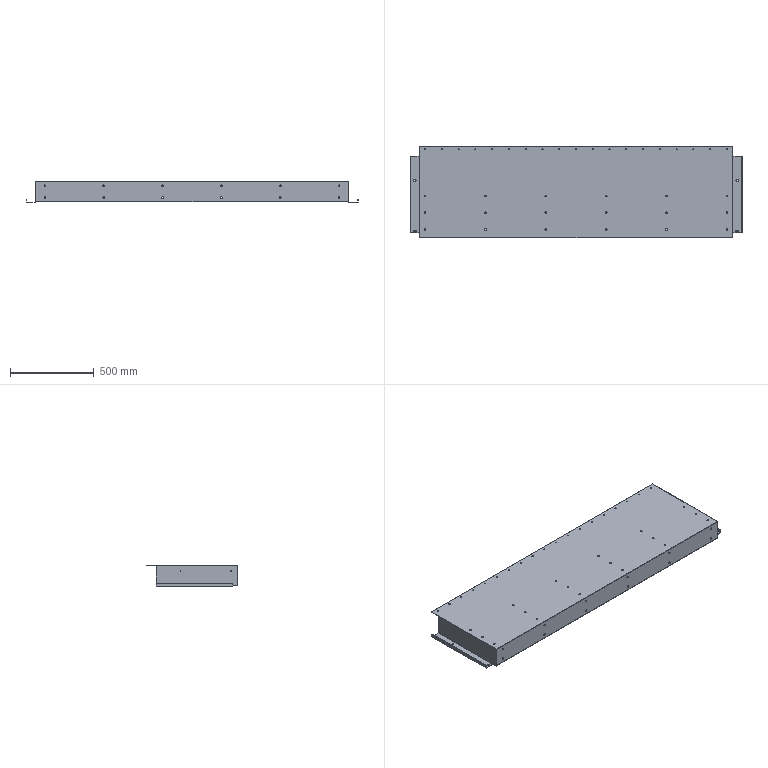Part | STEP file | SX-003-01 | 1 solid | 246 faces | box 1980 x 548 x 125 mm | volume 2956107 mm3 | cylinder 150 | plane 94 | spline 2 | commonest cylinder face diameters 7 x38 10 x36 5.4 x24 10.5 x24 8 x12 0.4 x8